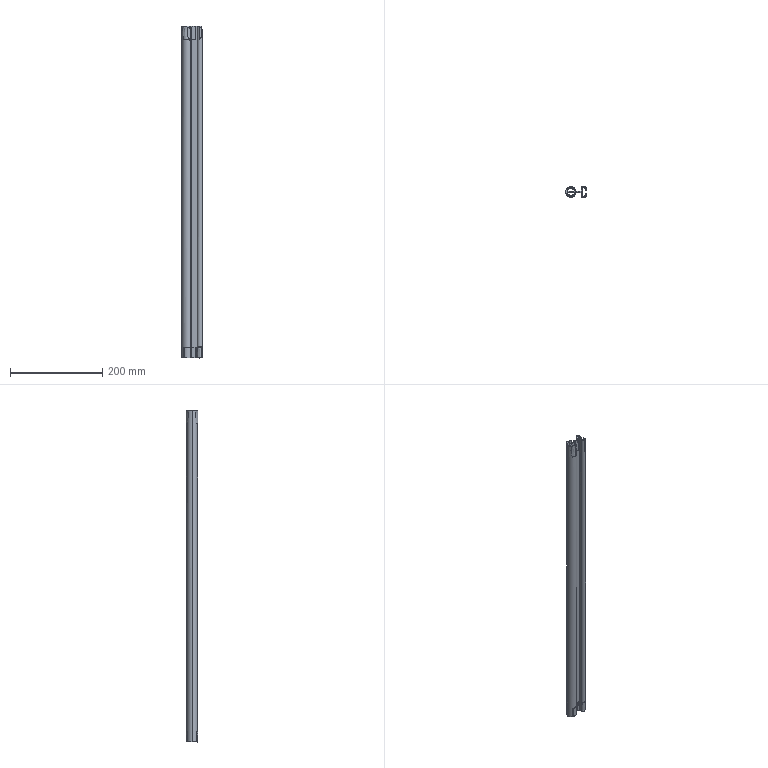Part | SolidWorks | features BaseBody 1 | 1 solid | 304 faces | box 44.505 x 24.701 x 719.001 mm | volume 253563 mm3 | spline 122 | cylinder 80 | plane 78 | cone 14 | torus 10 | commonest cylinder face diameters 0.9 x10 2 x8 1 x6 1.2 x6 10 x6 3.442 x4